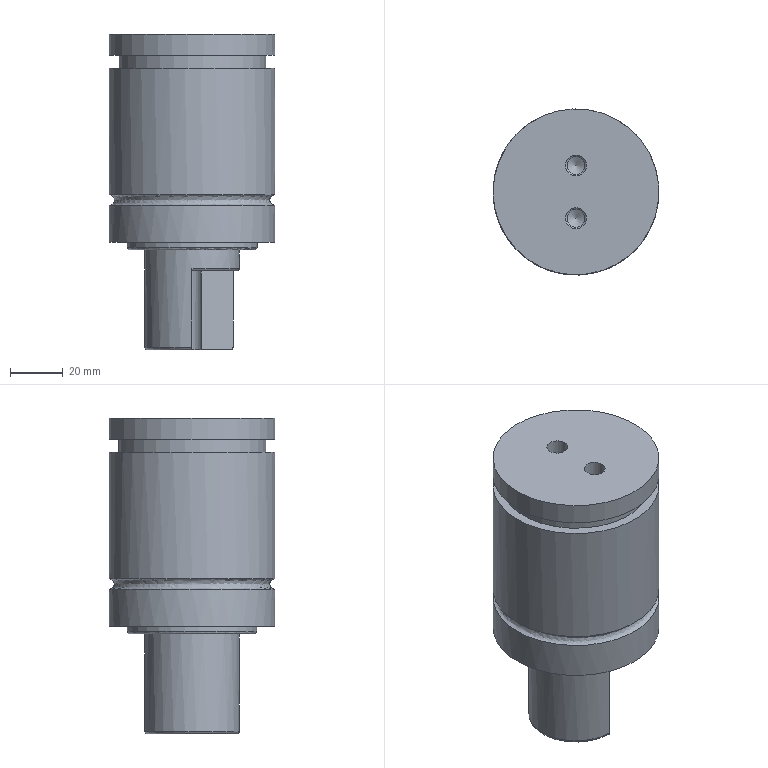Part | STEP file | GSV170-7_id1178_x_t | 1 solid | 166 faces | box 63 x 63 x 120 mm | volume 273871 mm3 | other 83 | plane 55 | cylinder 18 | cone 6 | torus 3 | spline 1 | commonest cylinder face diameters 63 x7 6.8 x3 8 x3 0.6 x1 3 x1 36 x1